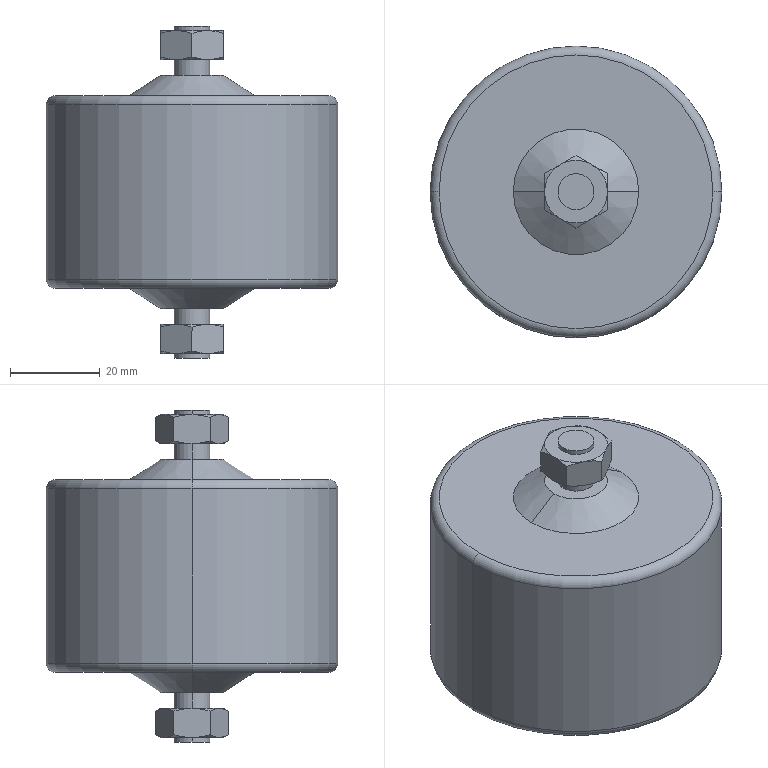Part | STEP file | JAJ-65_caster | 1 solid | 66 faces | box 65 x 65 x 74 mm | volume 148221 mm3 | plane 28 | cone 24 | cylinder 10 | torus 4 | commonest cylinder face diameters 8 x8 65 x2